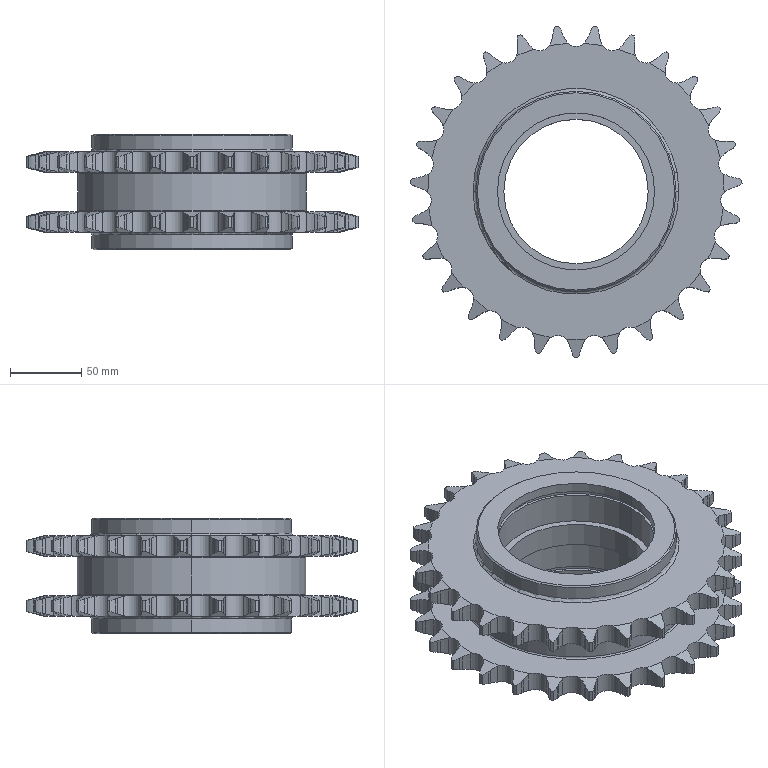Part | STEP file | 03-Driven sprocket 2 | 1 solid | 588 faces | box 232.271 x 231.883 x 81 mm | volume 1194859 mm3 | cylinder 344 | plane 120 | cone 116 | torus 8 | commonest cylinder face diameters 26.077 x108 41.357 x108 15.957 x54 232.551 x54 110 x8 114 x4